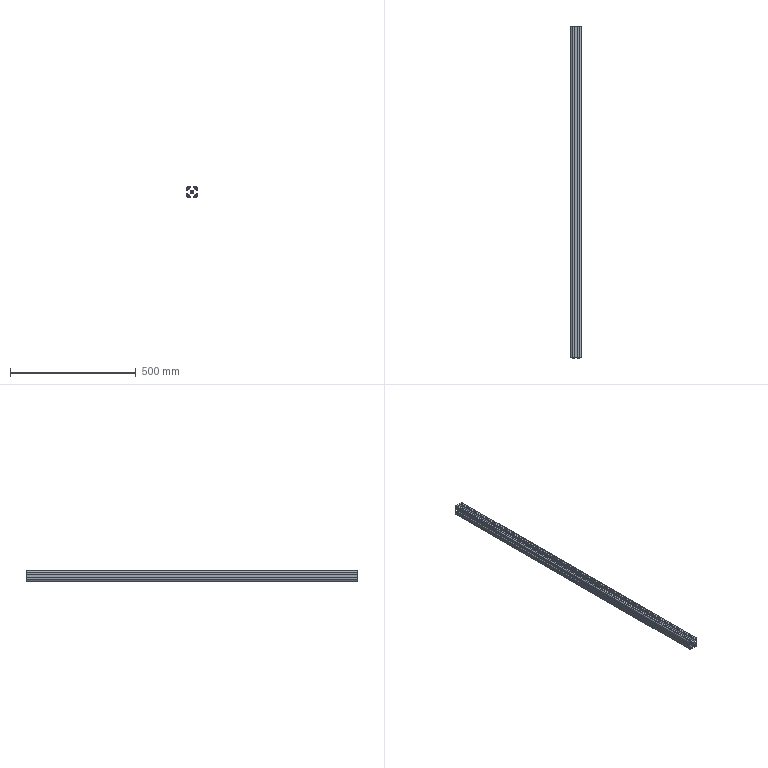Part | 1 solid | 104 faces | box 40 x 1319 x 40 mm | volume 760608 mm3 | plane 94 | cylinder 10 | commonest cylinder face diameters 5 x4 9 x4 6.8 x2